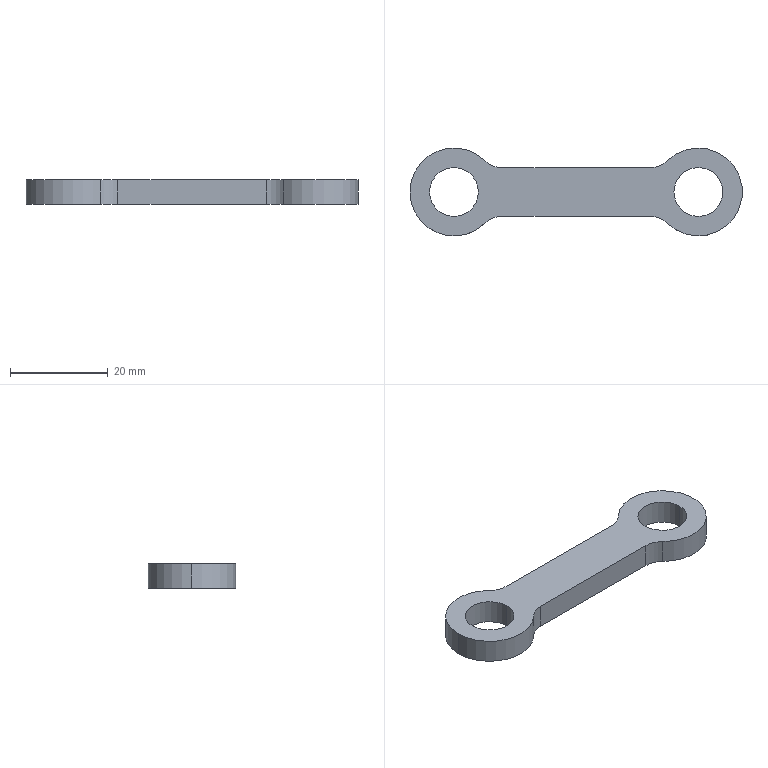Part | SolidWorks | features Extrusion 1 | 1 solid | 15 faces | box 68 x 18 x 5 mm | volume 3421 mm3 | cylinder 11 | plane 4 | commonest cylinder face diameters 10 x8 18 x3
STEP:
#1=CARTESIAN_POINT('',(45.,0.,5.));
#2=VERTEX_POINT('',#1);
#3=CARTESIAN_POINT('',(55.,0.,5.));
#4=VERTEX_POINT('',#3);
#5=CARTESIAN_POINT('',(50.,0.,5.));
#6=DIRECTION('',(0.,0.,1.));
#7=DIRECTION('',(1.,0.,0.));
#8=AXIS2_PLACEMENT_3D('',#5,#6,#7);
#9=CIRCLE('',#8,5.);
#10=EDGE_CURVE('',#2,#4,#9,.T.);
#11=ORIENTED_EDGE('',*,*,#10,.T.);
#12=CARTESIAN_POINT('',(55.,0.,0.));
#13=VERTEX_POINT('',#12);
#14=CARTESIAN_POINT('',(55.,0.,5.));
#15=DIRECTION('',(0.,0.,-1.));
#16=VECTOR('',#15,1000.);
#17=LINE('',#14,#16);
#18=EDGE_CURVE('',#4,#13,#17,.T.);
#19=ORIENTED_EDGE('',*,*,#18,.T.);
#20=CARTESIAN_POINT('',(45.,0.,0.));
#21=VERTEX_POINT('',#20);
#22=CARTESIAN_POINT('',(50.,0.,0.));
#23=DIRECTION('',(0.,0.,1.));
#24=DIRECTION('',(1.,0.,0.));
#25=AXIS2_PLACEMENT_3D('',#22,#23,#24);
#26=CIRCLE('',#25,5.);
#27=EDGE_CURVE('',#21,#13,#26,.T.);
#28=ORIENTED_EDGE('',*,*,#27,.F.);
#29=CARTESIAN_POINT('',(45.,0.,5.));
#30=DIRECTION('',(0.,0.,-1.));
#31=VECTOR('',#30,1000.);
#32=LINE('',#29,#31);
#33=EDGE_CURVE('',#2,#21,#32,.T.);
#34=ORIENTED_EDGE('',*,*,#33,.F.);
#35=EDGE_LOOP('',(#11,#19,#28,#34));
#36=FACE_OUTER_BOUND('',#35,.T.);
#37=CARTESIAN_POINT('',(50.,0.,5.));
#38=DIRECTION('',(0.,0.,-1.));
#39=DIRECTION('',(-1.,0.,0.));
#40=AXIS2_PLACEMENT_3D('',#37,#38,#39);
#41=CYLINDRICAL_SURFACE('',#40,5.);
#42=ADVANCED_FACE('',(#36),#41,.F.);
#43=CARTESIAN_POINT('',(-5.,0.,5.));
#44=VERTEX_POINT('',#43);
#45=CARTESIAN_POINT('',(5.,0.,5.));
#46=VERTEX_POINT('',#45);
#47=CARTESIAN_POINT('',(0.,0.,5.));
#48=DIRECTION('',(0.,0.,1.));
#49=DIRECTION('',(1.,0.,0.));
#50=AXIS2_PLACEMENT_3D('',#47,#48,#49);
#51=CIRCLE('',#50,5.);
#52=EDGE_CURVE('',#44,#46,#51,.T.);
#53=ORIENTED_EDGE('',*,*,#52,.T.);
#54=CARTESIAN_POINT('',(5.,0.,0.));
#55=VERTEX_POINT('',#54);
#56=CARTESIAN_POINT('',(5.,0.,5.));
#57=DIRECTION('',(0.,0.,-1.));
#58=VECTOR('',#57,1000.);
#59=LINE('',#56,#58);
#60=EDGE_CURVE('',#46,#55,#59,.T.);
#61=ORIENTED_EDGE('',*,*,#60,.T.);
#62=CARTESIAN_POINT('',(-5.,0.,0.));
#63=VERTEX_POINT('',#62);
#64=CARTESIAN_POINT('',(0.,0.,0.));
#65=DIRECTION('',(0.,0.,1.));
#66=DIRECTION('',(1.,0.,0.));
#67=AXIS2_PLACEMENT_3D('',#64,#65,#66);
#68=CIRCLE('',#67,5.);
#69=EDGE_CURVE('',#63,#55,#68,.T.);
#70=ORIENTED_EDGE('',*,*,#69,.F.);
#71=CARTESIAN_POINT('',(-5.,0.,5.));
#72=DIRECTION('',(0.,0.,-1.));
#73=VECTOR('',#72,1000.);
#74=LINE('',#71,#73);
#75=EDGE_CURVE('',#44,#63,#74,.T.);
#76=ORIENTED_EDGE('',*,*,#75,.F.);
#77=EDGE_LOOP('',(#53,#61,#70,#76));
#78=FACE_OUTER_BOUND('',#77,.T.);
#79=CARTESIAN_POINT('',(0.,0.,5.));
#80=DIRECTION('',(0.,0.,-1.));
#81=DIRECTION('',(-1.,0.,0.));
#82=AXIS2_PLACEMENT_3D('',#79,#80,#81);
#83=CYLINDRICAL_SURFACE('',#82,5.);
#84=ADVANCED_FACE('',(#78),#83,.F.);
#85=CARTESIAN_POINT('',(-9.,0.,5.));
#86=VERTEX_POINT('',#85);
#87=CARTESIAN_POINT('',(6.299,-6.429,5.));
#88=VERTEX_POINT('',#87);
#89=CARTESIAN_POINT('',(0.,0.,5.));
#90=DIRECTION('',(0.,0.,1.));
#91=DIRECTION('',(1.,0.,0.));
#92=AXIS2_PLACEMENT_3D('',#89,#90,#91);
#93=CIRCLE('',#92,9.);
#94=EDGE_CURVE('',#86,#88,#93,.T.);
#95=ORIENTED_EDGE('',*,*,#94,.F.);
#96=CARTESIAN_POINT('',(-9.,0.,0.));
#97=VERTEX_POINT('',#96);
#98=CARTESIAN_POINT('',(-9.,0.,5.));
#99=DIRECTION('',(0.,0.,-1.));
#100=VECTOR('',#99,1000.);
#101=LINE('',#98,#100);
#102=EDGE_CURVE('',#86,#97,#101,.T.);
#103=ORIENTED_EDGE('',*,*,#102,.T.);
#104=CARTESIAN_POINT('',(6.299,-6.429,0.));
#105=VERTEX_POINT('',#104);
#106=CARTESIAN_POINT('',(0.,0.,0.));
#107=DIRECTION('',(0.,0.,1.));
#108=DIRECTION('',(1.,0.,0.));
#109=AXIS2_PLACEMENT_3D('',#106,#107,#108);
#110=CIRCLE('',#109,9.);
#111=EDGE_CURVE('',#97,#105,#110,.T.);
#112=ORIENTED_EDGE('',*,*,#111,.T.);
#113=CARTESIAN_POINT('',(6.299,-6.429,5.));
#114=DIRECTION('',(0.,0.,-1.));
#115=VECTOR('',#114,1000.);
#116=LINE('',#113,#115);
#117=EDGE_CURVE('',#88,#105,#116,.T.);
#118=ORIENTED_EDGE('',*,*,#117,.F.);
#119=EDGE_LOOP('',(#95,#103,#112,#118));
#120=FACE_OUTER_BOUND('',#119,.T.);
#121=CARTESIAN_POINT('',(0.,0.,5.));
#122=DIRECTION('',(0.,0.,-1.));
#123=DIRECTION('',(-1.,0.,0.));
#124=AXIS2_PLACEMENT_3D('',#121,#122,#123);
#125=CYLINDRICAL_SURFACE('',#124,9.);
#126=ADVANCED_FACE('',(#120),#125,.T.);
#127=ORIENTED_EDGE('',*,*,#52,.F.);
#128=CARTESIAN_POINT('',(0.,0.,5.));
#129=DIRECTION('',(0.,0.,1.));
#130=DIRECTION('',(1.,0.,0.));
#131=AXIS2_PLACEMENT_3D('',#128,#129,#130);
#132=CIRCLE('',#131,5.);
#133=EDGE_CURVE('',#46,#44,#132,.T.);
#134=ORIENTED_EDGE('',*,*,#133,.F.);
#135=EDGE_LOOP('',(#127,#134));
#136=FACE_BOUND('',#135,.T.);
#137=CARTESIAN_POINT('',(43.701,6.429,5.));
#138=VERTEX_POINT('',#137);
#139=CARTESIAN_POINT('',(40.202,5.,5.));
#140=VERTEX_POINT('',#139);
#141=CARTESIAN_POINT('',(40.202,10.,5.));
#142=DIRECTION('',(0.,0.,-1.));
#143=DIRECTION('',(1.,0.,0.));
#144=AXIS2_PLACEMENT_3D('',#141,#142,#143);
#145=CIRCLE('',#144,5.);
#146=EDGE_CURVE('',#138,#140,#145,.T.);
#147=ORIENTED_EDGE('',*,*,#146,.T.);
#148=CARTESIAN_POINT('',(9.798,5.,5.));
#149=VERTEX_POINT('',#148);
#150=CARTESIAN_POINT('',(9.798,5.,5.));
#151=DIRECTION('',(-1.,0.,0.));
#152=VECTOR('',#151,1000.);
#153=LINE('',#150,#152);
#154=EDGE_CURVE('',#140,#149,#153,.T.);
#155=ORIENTED_EDGE('',*,*,#154,.T.);
#156=CARTESIAN_POINT('',(6.299,6.429,5.));
#157=VERTEX_POINT('',#156);
#158=CARTESIAN_POINT('',(9.798,10.,5.));
#159=DIRECTION('',(0.,0.,-1.));
#160=DIRECTION('',(-1.,0.,0.));
#161=AXIS2_PLACEMENT_3D('',#158,#159,#160);
#162=CIRCLE('',#161,5.);
#163=EDGE_CURVE('',#149,#157,#162,.T.);
#164=ORIENTED_EDGE('',*,*,#163,.T.);
#165=CARTESIAN_POINT('',(0.,0.,5.));
#166=DIRECTION('',(0.,0.,1.));
#167=DIRECTION('',(1.,0.,0.));
#168=AXIS2_PLACEMENT_3D('',#165,#166,#167);
#169=CIRCLE('',#168,9.);
#170=EDGE_CURVE('',#157,#86,#169,.T.);
#171=ORIENTED_EDGE('',*,*,#170,.T.);
#172=ORIENTED_EDGE('',*,*,#94,.T.);
#173=CARTESIAN_POINT('',(9.798,-5.,5.));
#174=VERTEX_POINT('',#173);
#175=CARTESIAN_POINT('',(9.798,-10.,5.));
#176=DIRECTION('',(0.,0.,-1.));
#177=DIRECTION('',(1.,0.,0.));
#178=AXIS2_PLACEMENT_3D('',#175,#176,#177);
#179=CIRCLE('',#178,5.);
#180=EDGE_CURVE('',#88,#174,#179,.T.);
#181=ORIENTED_EDGE('',*,*,#180,.T.);
#182=CARTESIAN_POINT('',(40.202,-5.,5.));
#183=VERTEX_POINT('',#182);
#184=CARTESIAN_POINT('',(9.798,-5.,5.));
#185=DIRECTION('',(1.,0.,0.));
#186=VECTOR('',#185,1000.);
#187=LINE('',#184,#186);
#188=EDGE_CURVE('',#174,#183,#187,.T.);
#189=ORIENTED_EDGE('',*,*,#188,.T.);
#190=CARTESIAN_POINT('',(43.701,-6.429,5.));
#191=VERTEX_POINT('',#190);
#192=CARTESIAN_POINT('',(40.202,-10.,5.));
#193=DIRECTION('',(0.,0.,-1.));
#194=DIRECTION('',(-1.,0.,0.));
#195=AXIS2_PLACEMENT_3D('',#192,#193,#194);
#196=CIRCLE('',#195,5.);
#197=EDGE_CURVE('',#183,#191,#196,.T.);
#198=ORIENTED_EDGE('',*,*,#197,.T.);
#199=CARTESIAN_POINT('',(50.,0.,5.));
#200=DIRECTION('',(0.,0.,1.));
#201=DIRECTION('',(1.,0.,0.));
#202=AXIS2_PLACEMENT_3D('',#199,#200,#201);
#203=CIRCLE('',#202,9.);
#204=EDGE_CURVE('',#191,#138,#203,.T.);
#205=ORIENTED_EDGE('',*,*,#204,.T.);
#206=EDGE_LOOP('',(#147,#155,#164,#171,#172,#181,#189,#198,#205));
#207=FACE_OUTER_BOUND('',#206,.T.);
#208=ORIENTED_EDGE('',*,*,#10,.F.);
#209=CARTESIAN_POINT('',(50.,0.,5.));
#210=DIRECTION('',(0.,0.,1.));
#211=DIRECTION('',(1.,0.,0.));
#212=AXIS2_PLACEMENT_3D('',#209,#210,#211);
#213=CIRCLE('',#212,5.);
#214=EDGE_CURVE('',#4,#2,#213,.T.);
#215=ORIENTED_EDGE('',*,*,#214,.F.);
#216=EDGE_LOOP('',(#208,#215));
#217=FACE_BOUND('',#216,.T.);
#218=CARTESIAN_POINT('',(40.202,10.,5.));
#219=DIRECTION('',(0.,0.,1.));
#220=DIRECTION('',(1.,0.,0.));
#221=AXIS2_PLACEMENT_3D('',#218,#219,#220);
#222=PLANE('',#221);
#223=ADVANCED_FACE('',(#136,#207,#217),#222,.T.);
#224=CARTESIAN_POINT('',(43.701,6.429,0.));
#225=VERTEX_POINT('',#224);
#226=CARTESIAN_POINT('',(40.202,5.,0.));
#227=VERTEX_POINT('',#226);
#228=CARTESIAN_POINT('',(40.202,10.,0.));
#229=DIRECTION('',(0.,0.,-1.));
#230=DIRECTION('',(1.,0.,0.));
#231=AXIS2_PLACEMENT_3D('',#228,#229,#230);
#232=CIRCLE('',#231,5.);
#233=EDGE_CURVE('',#225,#227,#232,.T.);
#234=ORIENTED_EDGE('',*,*,#233,.F.);
#235=CARTESIAN_POINT('',(43.701,-6.429,0.));
#236=VERTEX_POINT('',#235);
#237=CARTESIAN_POINT('',(50.,0.,0.));
#238=DIRECTION('',(0.,0.,1.));
#239=DIRECTION('',(1.,0.,0.));
#240=AXIS2_PLACEMENT_3D('',#237,#238,#239);
#241=CIRCLE('',#240,9.);
#242=EDGE_CURVE('',#236,#225,#241,.T.);
#243=ORIENTED_EDGE('',*,*,#242,.F.);
#244=CARTESIAN_POINT('',(40.202,-5.,0.));
#245=VERTEX_POINT('',#244);
#246=CARTESIAN_POINT('',(40.202,-10.,0.));
#247=DIRECTION('',(0.,0.,-1.));
#248=DIRECTION('',(-1.,0.,0.));
#249=AXIS2_PLACEMENT_3D('',#246,#247,#248);
#250=CIRCLE('',#249,5.);
#251=EDGE_CURVE('',#245,#236,#250,.T.);
#252=ORIENTED_EDGE('',*,*,#251,.F.);
#253=CARTESIAN_POINT('',(9.798,-5.,0.));
#254=VERTEX_POINT('',#253);
#255=CARTESIAN_POINT('',(9.798,-5.,0.));
#256=DIRECTION('',(1.,0.,0.));
#257=VECTOR('',#256,1000.);
#258=LINE('',#255,#257);
#259=EDGE_CURVE('',#254,#245,#258,.T.);
#260=ORIENTED_EDGE('',*,*,#259,.F.);
#261=CARTESIAN_POINT('',(9.798,-10.,0.));
#262=DIRECTION('',(0.,0.,-1.));
#263=DIRECTION('',(1.,0.,0.));
#264=AXIS2_PLACEMENT_3D('',#261,#262,#263);
#265=CIRCLE('',#264,5.);
#266=EDGE_CURVE('',#105,#254,#265,.T.);
#267=ORIENTED_EDGE('',*,*,#266,.F.);
#268=ORIENTED_EDGE('',*,*,#111,.F.);
#269=CARTESIAN_POINT('',(6.299,6.429,0.));
#270=VERTEX_POINT('',#269);
#271=CARTESIAN_POINT('',(0.,0.,0.));
#272=DIRECTION('',(0.,0.,1.));
#273=DIRECTION('',(1.,0.,0.));
#274=AXIS2_PLACEMENT_3D('',#271,#272,#273);
#275=CIRCLE('',#274,9.);
#276=EDGE_CURVE('',#270,#97,#275,.T.);
#277=ORIENTED_EDGE('',*,*,#276,.F.);
#278=CARTESIAN_POINT('',(9.798,5.,0.));
#279=VERTEX_POINT('',#278);
#280=CARTESIAN_POINT('',(9.798,10.,0.));
#281=DIRECTION('',(0.,0.,-1.));
#282=DIRECTION('',(-1.,0.,0.));
#283=AXIS2_PLACEMENT_3D('',#280,#281,#282);
#284=CIRCLE('',#283,5.);
#285=EDGE_CURVE('',#279,#270,#284,.T.);
#286=ORIENTED_EDGE('',*,*,#285,.F.);
#287=CARTESIAN_POINT('',(9.798,5.,0.));
#288=DIRECTION('',(-1.,0.,0.));
#289=VECTOR('',#288,1000.);
#290=LINE('',#287,#289);
#291=EDGE_CURVE('',#227,#279,#290,.T.);
#292=ORIENTED_EDGE('',*,*,#291,.F.);
#293=EDGE_LOOP('',(#234,#243,#252,#260,#267,#268,#277,#286,#292));
#294=FACE_OUTER_BOUND('',#293,.T.);
#295=ORIENTED_EDGE('',*,*,#69,.T.);
#296=CARTESIAN_POINT('',(0.,0.,0.));
#297=DIRECTION('',(0.,0.,1.));
#298=DIRECTION('',(1.,0.,0.));
#299=AXIS2_PLACEMENT_3D('',#296,#297,#298);
#300=CIRCLE('',#299,5.);
#301=EDGE_CURVE('',#55,#63,#300,.T.);
#302=ORIENTED_EDGE('',*,*,#301,.T.);
#303=EDGE_LOOP('',(#295,#302));
#304=FACE_BOUND('',#303,.T.);
#305=ORIENTED_EDGE('',*,*,#27,.T.);
#306=CARTESIAN_POINT('',(50.,0.,0.));
#307=DIRECTION('',(0.,0.,1.));
#308=DIRECTION('',(1.,0.,0.));
#309=AXIS2_PLACEMENT_3D('',#306,#307,#308);
#310=CIRCLE('',#309,5.);
#311=EDGE_CURVE('',#13,#21,#310,.T.);
#312=ORIENTED_EDGE('',*,*,#311,.T.);
#313=EDGE_LOOP('',(#305,#312));
#314=FACE_BOUND('',#313,.T.);
#315=CARTESIAN_POINT('',(40.202,10.,0.));
#316=DIRECTION('',(0.,0.,1.));
#317=DIRECTION('',(1.,0.,0.));
#318=AXIS2_PLACEMENT_3D('',#315,#316,#317);
#319=PLANE('',#318);
#320=ADVANCED_FACE('',(#294,#304,#314),#319,.F.);
#321=ORIENTED_EDGE('',*,*,#233,.T.);
#322=CARTESIAN_POINT('',(40.202,5.,5.));
#323=DIRECTION('',(0.,0.,-1.));
#324=VECTOR('',#323,1000.);
#325=LINE('',#322,#324);
#326=EDGE_CURVE('',#140,#227,#325,.T.);
#327=ORIENTED_EDGE('',*,*,#326,.F.);
#328=ORIENTED_EDGE('',*,*,#146,.F.);
#329=CARTESIAN_POINT('',(43.701,6.429,5.));
#330=DIRECTION('',(0.,0.,-1.));
#331=VECTOR('',#330,1000.);
#332=LINE('',#329,#331);
#333=EDGE_CURVE('',#138,#225,#332,.T.);
#334=ORIENTED_EDGE('',*,*,#333,.T.);
#335=EDGE_LOOP('',(#321,#327,#328,#334));
#336=FACE_OUTER_BOUND('',#335,.T.);
#337=CARTESIAN_POINT('',(40.202,10.,5.));
#338=DIRECTION('',(0.,0.,-1.));
#339=DIRECTION('',(-1.,0.,0.));
#340=AXIS2_PLACEMENT_3D('',#337,#338,#339);
#341=CYLINDRICAL_SURFACE('',#340,5.);
#342=ADVANCED_FACE('',(#336),#341,.F.);
#343=ORIENTED_EDGE('',*,*,#291,.T.);
#344=CARTESIAN_POINT('',(9.798,5.,5.));
#345=DIRECTION('',(0.,0.,-1.));
#346=VECTOR('',#345,1000.);
#347=LINE('',#344,#346);
#348=EDGE_CURVE('',#149,#279,#347,.T.);
#349=ORIENTED_EDGE('',*,*,#348,.F.);
#350=ORIENTED_EDGE('',*,*,#154,.F.);
#351=ORIENTED_EDGE('',*,*,#326,.T.);
#352=EDGE_LOOP('',(#343,#349,#350,#351));
#353=FACE_OUTER_BOUND('',#352,.T.);
#354=CARTESIAN_POINT('',(9.798,5.,5.));
#355=DIRECTION('',(0.,-1.,0.));
#356=DIRECTION('',(1.,0.,0.));
#357=AXIS2_PLACEMENT_3D('',#354,#355,#356);
#358=PLANE('',#357);
#359=ADVANCED_FACE('',(#353),#358,.F.);
#360=ORIENTED_EDGE('',*,*,#285,.T.);
#361=CARTESIAN_POINT('',(6.299,6.429,5.));
#362=DIRECTION('',(0.,0.,-1.));
#363=VECTOR('',#362,1000.);
#364=LINE('',#361,#363);
#365=EDGE_CURVE('',#157,#270,#364,.T.);
#366=ORIENTED_EDGE('',*,*,#365,.F.);
#367=ORIENTED_EDGE('',*,*,#163,.F.);
#368=ORIENTED_EDGE('',*,*,#348,.T.);
#369=EDGE_LOOP('',(#360,#366,#367,#368));
#370=FACE_OUTER_BOUND('',#369,.T.);
#371=CARTESIAN_POINT('',(9.798,10.,5.));
#372=DIRECTION('',(0.,0.,-1.));
#373=DIRECTION('',(-1.,0.,0.));
#374=AXIS2_PLACEMENT_3D('',#371,#372,#373);
#375=CYLINDRICAL_SURFACE('',#374,5.);
#376=ADVANCED_FACE('',(#370),#375,.F.);
#377=ORIENTED_EDGE('',*,*,#102,.F.);
#378=ORIENTED_EDGE('',*,*,#170,.F.);
#379=ORIENTED_EDGE('',*,*,#365,.T.);
#380=ORIENTED_EDGE('',*,*,#276,.T.);
#381=EDGE_LOOP('',(#377,#378,#379,#380));
#382=FACE_OUTER_BOUND('',#381,.T.);
#383=CARTESIAN_POINT('',(0.,0.,5.));
#384=DIRECTION('',(0.,0.,-1.));
#385=DIRECTION('',(-1.,0.,0.));
#386=AXIS2_PLACEMENT_3D('',#383,#384,#385);
#387=CYLINDRICAL_SURFACE('',#386,9.);
#388=ADVANCED_FACE('',(#382),#387,.T.);
#389=ORIENTED_EDGE('',*,*,#266,.T.);
#390=CARTESIAN_POINT('',(9.798,-5.,5.));
#391=DIRECTION('',(0.,0.,-1.));
#392=VECTOR('',#391,1000.);
#393=LINE('',#390,#392);
#394=EDGE_CURVE('',#174,#254,#393,.T.);
#395=ORIENTED_EDGE('',*,*,#394,.F.);
#396=ORIENTED_EDGE('',*,*,#180,.F.);
#397=ORIENTED_EDGE('',*,*,#117,.T.);
#398=EDGE_LOOP('',(#389,#395,#396,#397));
#399=FACE_OUTER_BOUND('',#398,.T.);
#400=CARTESIAN_POINT('',(9.798,-10.,5.));
#401=DIRECTION('',(0.,0.,-1.));
#402=DIRECTION('',(-1.,0.,0.));
#403=AXIS2_PLACEMENT_3D('',#400,#401,#402);
#404=CYLINDRICAL_SURFACE('',#403,5.);
#405=ADVANCED_FACE('',(#399),#404,.F.);
#406=ORIENTED_EDGE('',*,*,#259,.T.);
#407=CARTESIAN_POINT('',(40.202,-5.,5.));
#408=DIRECTION('',(0.,0.,-1.));
#409=VECTOR('',#408,1000.);
#410=LINE('',#407,#409);
#411=EDGE_CURVE('',#183,#245,#410,.T.);
#412=ORIENTED_EDGE('',*,*,#411,.F.);
#413=ORIENTED_EDGE('',*,*,#188,.F.);
#414=ORIENTED_EDGE('',*,*,#394,.T.);
#415=EDGE_LOOP('',(#406,#412,#413,#414));
#416=FACE_OUTER_BOUND('',#415,.T.);
#417=CARTESIAN_POINT('',(9.798,-5.,5.));
#418=DIRECTION('',(0.,1.,0.));
#419=DIRECTION('',(-1.,0.,0.));
#420=AXIS2_PLACEMENT_3D('',#417,#418,#419);
#421=PLANE('',#420);
#422=ADVANCED_FACE('',(#416),#421,.F.);
#423=ORIENTED_EDGE('',*,*,#251,.T.);
#424=CARTESIAN_POINT('',(43.701,-6.429,5.));
#425=DIRECTION('',(0.,0.,-1.));
#426=VECTOR('',#425,1000.);
#427=LINE('',#424,#426);
#428=EDGE_CURVE('',#191,#236,#427,.T.);
#429=ORIENTED_EDGE('',*,*,#428,.F.);
#430=ORIENTED_EDGE('',*,*,#197,.F.);
#431=ORIENTED_EDGE('',*,*,#411,.T.);
#432=EDGE_LOOP('',(#423,#429,#430,#431));
#433=FACE_OUTER_BOUND('',#432,.T.);
#434=CARTESIAN_POINT('',(40.202,-10.,5.));
#435=DIRECTION('',(0.,0.,-1.));
#436=DIRECTION('',(-1.,0.,0.));
#437=AXIS2_PLACEMENT_3D('',#434,#435,#436);
#438=CYLINDRICAL_SURFACE('',#437,5.);
#439=ADVANCED_FACE('',(#433),#438,.F.);
#440=ORIENTED_EDGE('',*,*,#242,.T.);
#441=ORIENTED_EDGE('',*,*,#333,.F.);
#442=ORIENTED_EDGE('',*,*,#204,.F.);
#443=ORIENTED_EDGE('',*,*,#428,.T.);
#444=EDGE_LOOP('',(#440,#441,#442,#443));
#445=FACE_OUTER_BOUND('',#444,.T.);
#446=CARTESIAN_POINT('',(50.,0.,5.));
#447=DIRECTION('',(0.,0.,-1.));
#448=DIRECTION('',(-1.,0.,0.));
#449=AXIS2_PLACEMENT_3D('',#446,#447,#448);
#450=CYLINDRICAL_SURFACE('',#449,9.);
#451=ADVANCED_FACE('',(#445),#450,.T.);
#452=ORIENTED_EDGE('',*,*,#60,.F.);
#453=ORIENTED_EDGE('',*,*,#133,.T.);
#454=ORIENTED_EDGE('',*,*,#75,.T.);
#455=ORIENTED_EDGE('',*,*,#301,.F.);
#456=EDGE_LOOP('',(#452,#453,#454,#455));
#457=FACE_OUTER_BOUND('',#456,.T.);
#458=CARTESIAN_POINT('',(0.,0.,5.));
#459=DIRECTION('',(0.,0.,-1.));
#460=DIRECTION('',(-1.,0.,0.));
#461=AXIS2_PLACEMENT_3D('',#458,#459,#460);
#462=CYLINDRICAL_SURFACE('',#461,5.);
#463=ADVANCED_FACE('',(#457),#462,.F.);
#464=ORIENTED_EDGE('',*,*,#18,.F.);
#465=ORIENTED_EDGE('',*,*,#214,.T.);
#466=ORIENTED_EDGE('',*,*,#33,.T.);
#467=ORIENTED_EDGE('',*,*,#311,.F.);
#468=EDGE_LOOP('',(#464,#465,#466,#467));
#469=FACE_OUTER_BOUND('',#468,.T.);
#470=CARTESIAN_POINT('',(50.,0.,5.));
#471=DIRECTION('',(0.,0.,-1.));
#472=DIRECTION('',(-1.,0.,0.));
#473=AXIS2_PLACEMENT_3D('',#470,#471,#472);
#474=CYLINDRICAL_SURFACE('',#473,5.);
#475=ADVANCED_FACE('',(#469),#474,.F.);
#476=CLOSED_SHELL('',(#42,#84,#126,#223,#320,#342,#359,#376,#388,#405,#422,#439,#451,#463,#475));
#477=MANIFOLD_SOLID_BREP('',#476);
#478=CARTESIAN_POINT('',(0.,0.,0.));
#479=DIRECTION('',(0.,0.,1.));
#480=DIRECTION('',(1.,0.,0.));
#481=AXIS2_PLACEMENT_3D('',#478,#479,#480);
#482=(LENGTH_UNIT()NAMED_UNIT(*)SI_UNIT(.MILLI.,.METRE.));
#483=UNCERTAINTY_MEASURE_WITH_UNIT(LENGTH_MEASURE(0.00001),#482,'','');
#484=(NAMED_UNIT(*)PLANE_ANGLE_UNIT()SI_UNIT($,.RADIAN.));
#485=(NAMED_UNIT(*)SI_UNIT($,.STERADIAN.)SOLID_ANGLE_UNIT());
#486=(GEOMETRIC_REPRESENTATION_CONTEXT(3)GLOBAL_UNCERTAINTY_ASSIGNED_CONTEXT((#483))GLOBAL_UNIT_ASSIGNED_CONTEXT((#482,#484,#485))REPRESENTATION_CONTEXT('',''));
#487=ADVANCED_BREP_SHAPE_REPRESENTATION('',(#477,#481),#486);